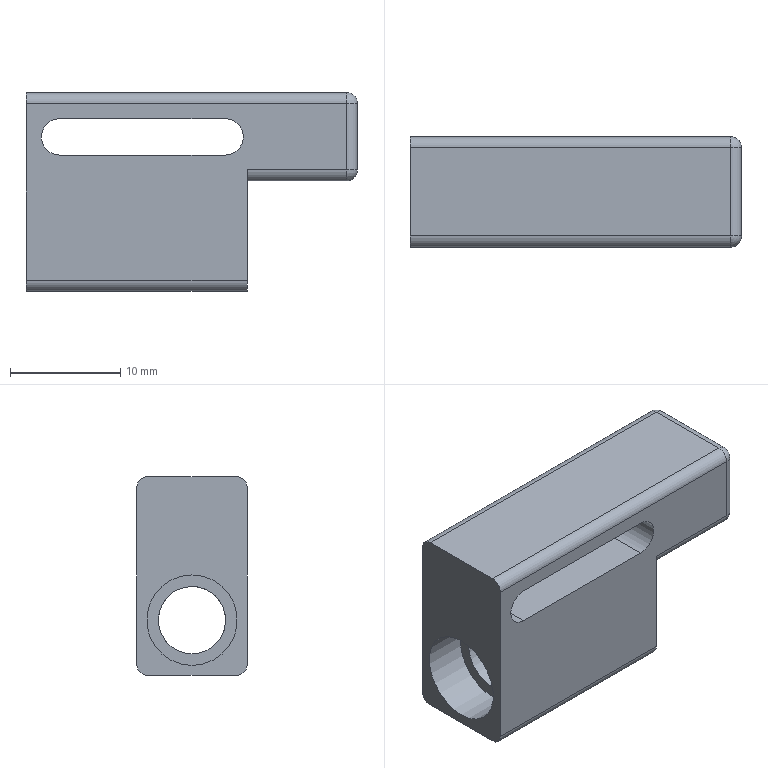Part | NX | 1 solid | 29 faces | box 30 x 10 x 18 mm | volume 3108 mm3 | cylinder 14 | plane 11 | sphere 4 | commonest cylinder face diameters 2 x10 3.3 x2 6.1 x1 8.2 x1
STEP:
#1=CARTESIAN_POINT('',(-11.,5.,-12.05));
#2=VERTEX_POINT('',#1);
#3=CARTESIAN_POINT('',(-11.,5.,-9.));
#4=DIRECTION('',(-1.,0.,0.));
#5=DIRECTION('',(0.,0.,-1.));
#6=AXIS2_PLACEMENT_3D('',#3,#4,#5);
#7=CIRCLE('',#6,3.05);
#8=EDGE_CURVE('',#2,#2,#7,.T.);
#9=ORIENTED_EDGE('',*,*,#8,.F.);
#10=EDGE_LOOP('',(#9));
#11=FACE_BOUND('',#10,.T.);
#12=CARTESIAN_POINT('',(-11.,5.,-13.1));
#13=VERTEX_POINT('',#12);
#14=CARTESIAN_POINT('',(-11.,5.,-9.));
#15=DIRECTION('',(1.,0.,0.));
#16=DIRECTION('',(0.,0.,-1.));
#17=AXIS2_PLACEMENT_3D('',#14,#15,#16);
#18=CIRCLE('',#17,4.1);
#19=EDGE_CURVE('',#13,#13,#18,.T.);
#20=ORIENTED_EDGE('',*,*,#19,.F.);
#21=EDGE_LOOP('',(#20));
#22=FACE_BOUND('',#21,.T.);
#23=CARTESIAN_POINT('',(-11.,5.,-9.));
#24=DIRECTION('',(1.,0.,0.));
#25=DIRECTION('',(0.,0.,-1.));
#26=AXIS2_PLACEMENT_3D('',#23,#24,#25);
#27=PLANE('',#26);
#28=ADVANCED_FACE('',(#11,#22),#27,.F.);
#29=CARTESIAN_POINT('',(5.,0.,-13.));
#30=VERTEX_POINT('',#29);
#31=CARTESIAN_POINT('',(5.,1.,-14.));
#32=VERTEX_POINT('',#31);
#33=CARTESIAN_POINT('',(5.,1.,-13.));
#34=DIRECTION('',(1.,0.,0.));
#35=DIRECTION('',(0.,-1.,0.));
#36=AXIS2_PLACEMENT_3D('',#33,#34,#35);
#37=CIRCLE('',#36,1.);
#38=EDGE_CURVE('',#30,#32,#37,.T.);
#39=ORIENTED_EDGE('',*,*,#38,.F.);
#40=CARTESIAN_POINT('',(-15.,0.,-13.));
#41=VERTEX_POINT('',#40);
#42=CARTESIAN_POINT('',(5.,0.,-13.));
#43=DIRECTION('',(1.,0.,0.));
#44=VECTOR('',#43,1000.);
#45=LINE('',#42,#44);
#46=EDGE_CURVE('',#41,#30,#45,.T.);
#47=ORIENTED_EDGE('',*,*,#46,.F.);
#48=CARTESIAN_POINT('',(-15.,1.,-14.));
#49=VERTEX_POINT('',#48);
#50=CARTESIAN_POINT('',(-15.,1.,-13.));
#51=DIRECTION('',(-1.,0.,0.));
#52=DIRECTION('',(0.,0.,-1.));
#53=AXIS2_PLACEMENT_3D('',#50,#51,#52);
#54=CIRCLE('',#53,1.);
#55=EDGE_CURVE('',#49,#41,#54,.T.);
#56=ORIENTED_EDGE('',*,*,#55,.F.);
#57=CARTESIAN_POINT('',(-15.,1.,-14.));
#58=DIRECTION('',(-1.,0.,0.));
#59=VECTOR('',#58,1000.);
#60=LINE('',#57,#59);
#61=EDGE_CURVE('',#32,#49,#60,.T.);
#62=ORIENTED_EDGE('',*,*,#61,.F.);
#63=EDGE_LOOP('',(#39,#47,#56,#62));
#64=FACE_BOUND('',#63,.T.);
#65=CARTESIAN_POINT('',(0.,1.,-13.));
#66=DIRECTION('',(1.,0.,0.));
#67=DIRECTION('',(0.,0.,-1.));
#68=AXIS2_PLACEMENT_3D('',#65,#66,#67);
#69=CYLINDRICAL_SURFACE('',#68,1.);
#70=ADVANCED_FACE('',(#64),#69,.T.);
#71=CARTESIAN_POINT('',(-15.,10.,-13.));
#72=VERTEX_POINT('',#71);
#73=CARTESIAN_POINT('',(-15.,9.,-14.));
#74=VERTEX_POINT('',#73);
#75=CARTESIAN_POINT('',(-15.,9.,-13.));
#76=DIRECTION('',(-1.,0.,0.));
#77=DIRECTION('',(0.,0.,-1.));
#78=AXIS2_PLACEMENT_3D('',#75,#76,#77);
#79=CIRCLE('',#78,1.);
#80=EDGE_CURVE('',#72,#74,#79,.T.);
#81=ORIENTED_EDGE('',*,*,#80,.F.);
#82=CARTESIAN_POINT('',(5.,10.,-13.));
#83=VERTEX_POINT('',#82);
#84=CARTESIAN_POINT('',(0.,10.,-13.));
#85=DIRECTION('',(-1.,0.,0.));
#86=VECTOR('',#85,1000.);
#87=LINE('',#84,#86);
#88=EDGE_CURVE('',#83,#72,#87,.T.);
#89=ORIENTED_EDGE('',*,*,#88,.F.);
#90=CARTESIAN_POINT('',(5.,9.,-14.));
#91=VERTEX_POINT('',#90);
#92=CARTESIAN_POINT('',(5.,9.,-13.));
#93=DIRECTION('',(1.,0.,0.));
#94=DIRECTION('',(0.,-1.,0.));
#95=AXIS2_PLACEMENT_3D('',#92,#93,#94);
#96=CIRCLE('',#95,1.);
#97=EDGE_CURVE('',#91,#83,#96,.T.);
#98=ORIENTED_EDGE('',*,*,#97,.F.);
#99=CARTESIAN_POINT('',(0.,9.,-14.));
#100=DIRECTION('',(1.,0.,0.));
#101=VECTOR('',#100,1000.);
#102=LINE('',#99,#101);
#103=EDGE_CURVE('',#74,#91,#102,.T.);
#104=ORIENTED_EDGE('',*,*,#103,.F.);
#105=EDGE_LOOP('',(#81,#89,#98,#104));
#106=FACE_BOUND('',#105,.T.);
#107=CARTESIAN_POINT('',(0.,9.,-13.));
#108=DIRECTION('',(1.,0.,0.));
#109=DIRECTION('',(0.,0.,-1.));
#110=AXIS2_PLACEMENT_3D('',#107,#108,#109);
#111=CYLINDRICAL_SURFACE('',#110,1.);
#112=ADVANCED_FACE('',(#106),#111,.T.);
#113=CARTESIAN_POINT('',(15.,1.,3.));
#114=VERTEX_POINT('',#113);
#115=CARTESIAN_POINT('',(14.,1.,4.));
#116=VERTEX_POINT('',#115);
#117=CARTESIAN_POINT('',(14.,1.,3.));
#118=DIRECTION('',(0.,-1.,0.));
#119=DIRECTION('',(0.,0.,-1.));
#120=AXIS2_PLACEMENT_3D('',#117,#118,#119);
#121=CIRCLE('',#120,1.);
#122=EDGE_CURVE('',#114,#116,#121,.T.);
#123=ORIENTED_EDGE('',*,*,#122,.T.);
#124=CARTESIAN_POINT('',(14.,0.,3.));
#125=VERTEX_POINT('',#124);
#126=CARTESIAN_POINT('',(14.,1.,3.));
#127=DIRECTION('',(-1.,0.,0.));
#128=DIRECTION('',(0.,0.,1.));
#129=AXIS2_PLACEMENT_3D('',#126,#127,#128);
#130=CIRCLE('',#129,1.);
#131=EDGE_CURVE('',#125,#116,#130,.T.);
#132=ORIENTED_EDGE('',*,*,#131,.F.);
#133=CARTESIAN_POINT('',(14.,1.,3.));
#134=DIRECTION('',(0.,0.,1.));
#135=DIRECTION('',(1.,0.,0.));
#136=AXIS2_PLACEMENT_3D('',#133,#134,#135);
#137=CIRCLE('',#136,1.);
#138=EDGE_CURVE('',#125,#114,#137,.T.);
#139=ORIENTED_EDGE('',*,*,#138,.T.);
#140=EDGE_LOOP('',(#123,#132,#139));
#141=FACE_BOUND('',#140,.T.);
#142=CARTESIAN_POINT('',(14.,1.,3.));
#143=DIRECTION('',(0.,0.,1.));
#144=DIRECTION('',(1.,0.,0.));
#145=AXIS2_PLACEMENT_3D('',#142,#143,#144);
#146=SPHERICAL_SURFACE('',#145,1.);
#147=ADVANCED_FACE('',(#141),#146,.T.);
#148=CARTESIAN_POINT('',(14.,0.,-3.));
#149=VERTEX_POINT('',#148);
#150=CARTESIAN_POINT('',(15.,1.,-3.));
#151=VERTEX_POINT('',#150);
#152=CARTESIAN_POINT('',(14.,1.,-3.));
#153=DIRECTION('',(0.,0.,1.));
#154=DIRECTION('',(1.,0.,0.));
#155=AXIS2_PLACEMENT_3D('',#152,#153,#154);
#156=CIRCLE('',#155,1.);
#157=EDGE_CURVE('',#149,#151,#156,.T.);
#158=ORIENTED_EDGE('',*,*,#157,.T.);
#159=CARTESIAN_POINT('',(15.,1.,-3.));
#160=DIRECTION('',(0.,0.,-1.));
#161=VECTOR('',#160,1000.);
#162=LINE('',#159,#161);
#163=EDGE_CURVE('',#114,#151,#162,.T.);
#164=ORIENTED_EDGE('',*,*,#163,.F.);
#165=ORIENTED_EDGE('',*,*,#138,.F.);
#166=CARTESIAN_POINT('',(14.,0.,3.));
#167=DIRECTION('',(0.,0.,1.));
#168=VECTOR('',#167,1000.);
#169=LINE('',#166,#168);
#170=EDGE_CURVE('',#149,#125,#169,.T.);
#171=ORIENTED_EDGE('',*,*,#170,.F.);
#172=EDGE_LOOP('',(#158,#164,#165,#171));
#173=FACE_BOUND('',#172,.T.);
#174=CARTESIAN_POINT('',(14.,1.,4.));
#175=DIRECTION('',(0.,0.,1.));
#176=DIRECTION('',(1.,0.,0.));
#177=AXIS2_PLACEMENT_3D('',#174,#175,#176);
#178=CYLINDRICAL_SURFACE('',#177,1.);
#179=ADVANCED_FACE('',(#173),#178,.T.);
#180=CARTESIAN_POINT('',(15.,9.,3.));
#181=VERTEX_POINT('',#180);
#182=CARTESIAN_POINT('',(14.,9.,4.));
#183=VERTEX_POINT('',#182);
#184=CARTESIAN_POINT('',(14.,9.,3.));
#185=DIRECTION('',(0.,-1.,0.));
#186=DIRECTION('',(0.,0.,-1.));
#187=AXIS2_PLACEMENT_3D('',#184,#185,#186);
#188=CIRCLE('',#187,1.);
#189=EDGE_CURVE('',#181,#183,#188,.T.);
#190=ORIENTED_EDGE('',*,*,#189,.T.);
#191=CARTESIAN_POINT('',(14.,10.,4.));
#192=DIRECTION('',(0.,1.,0.));
#193=VECTOR('',#192,1000.);
#194=LINE('',#191,#193);
#195=EDGE_CURVE('',#116,#183,#194,.T.);
#196=ORIENTED_EDGE('',*,*,#195,.F.);
#197=ORIENTED_EDGE('',*,*,#122,.F.);
#198=CARTESIAN_POINT('',(15.,10.,3.));
#199=DIRECTION('',(0.,-1.,0.));
#200=VECTOR('',#199,1000.);
#201=LINE('',#198,#200);
#202=EDGE_CURVE('',#181,#114,#201,.T.);
#203=ORIENTED_EDGE('',*,*,#202,.F.);
#204=EDGE_LOOP('',(#190,#196,#197,#203));
#205=FACE_BOUND('',#204,.T.);
#206=CARTESIAN_POINT('',(14.,10.,3.));
#207=DIRECTION('',(0.,-1.,0.));
#208=DIRECTION('',(0.,0.,-1.));
#209=AXIS2_PLACEMENT_3D('',#206,#207,#208);
#210=CYLINDRICAL_SURFACE('',#209,1.);
#211=ADVANCED_FACE('',(#205),#210,.T.);
#212=CARTESIAN_POINT('',(14.,1.,-4.));
#213=VERTEX_POINT('',#212);
#214=CARTESIAN_POINT('',(14.,1.,-3.));
#215=DIRECTION('',(1.,0.,0.));
#216=DIRECTION('',(0.,0.,-1.));
#217=AXIS2_PLACEMENT_3D('',#214,#215,#216);
#218=CIRCLE('',#217,1.);
#219=EDGE_CURVE('',#213,#149,#218,.F.);
#220=ORIENTED_EDGE('',*,*,#219,.F.);
#221=CARTESIAN_POINT('',(14.,1.,-3.));
#222=DIRECTION('',(0.,-1.,0.));
#223=DIRECTION('',(0.,0.,-1.));
#224=AXIS2_PLACEMENT_3D('',#221,#222,#223);
#225=CIRCLE('',#224,1.);
#226=EDGE_CURVE('',#213,#151,#225,.T.);
#227=ORIENTED_EDGE('',*,*,#226,.T.);
#228=ORIENTED_EDGE('',*,*,#157,.F.);
#229=EDGE_LOOP('',(#220,#227,#228));
#230=FACE_BOUND('',#229,.T.);
#231=CARTESIAN_POINT('',(14.,1.,-3.));
#232=DIRECTION('',(0.,0.,1.));
#233=DIRECTION('',(1.,0.,0.));
#234=AXIS2_PLACEMENT_3D('',#231,#232,#233);
#235=SPHERICAL_SURFACE('',#234,1.);
#236=ADVANCED_FACE('',(#230),#235,.T.);
#237=CARTESIAN_POINT('',(14.,10.,3.));
#238=VERTEX_POINT('',#237);
#239=CARTESIAN_POINT('',(14.,9.,3.));
#240=DIRECTION('',(0.,0.,-1.));
#241=DIRECTION('',(-1.,0.,0.));
#242=AXIS2_PLACEMENT_3D('',#239,#240,#241);
#243=CIRCLE('',#242,1.);
#244=EDGE_CURVE('',#181,#238,#243,.F.);
#245=ORIENTED_EDGE('',*,*,#244,.T.);
#246=CARTESIAN_POINT('',(14.,9.,3.));
#247=DIRECTION('',(1.,0.,0.));
#248=DIRECTION('',(0.,0.,-1.));
#249=AXIS2_PLACEMENT_3D('',#246,#247,#248);
#250=CIRCLE('',#249,1.);
#251=EDGE_CURVE('',#183,#238,#250,.F.);
#252=ORIENTED_EDGE('',*,*,#251,.F.);
#253=ORIENTED_EDGE('',*,*,#189,.F.);
#254=EDGE_LOOP('',(#245,#252,#253));
#255=FACE_BOUND('',#254,.T.);
#256=CARTESIAN_POINT('',(14.,9.,3.));
#257=DIRECTION('',(0.,0.,1.));
#258=DIRECTION('',(1.,0.,0.));
#259=AXIS2_PLACEMENT_3D('',#256,#257,#258);
#260=SPHERICAL_SURFACE('',#259,1.);
#261=ADVANCED_FACE('',(#255),#260,.T.);
#262=CARTESIAN_POINT('',(14.,9.,-4.));
#263=VERTEX_POINT('',#262);
#264=CARTESIAN_POINT('',(15.,9.,-3.));
#265=VERTEX_POINT('',#264);
#266=CARTESIAN_POINT('',(14.,9.,-3.));
#267=DIRECTION('',(0.,-1.,0.));
#268=DIRECTION('',(0.,0.,-1.));
#269=AXIS2_PLACEMENT_3D('',#266,#267,#268);
#270=CIRCLE('',#269,1.);
#271=EDGE_CURVE('',#263,#265,#270,.T.);
#272=ORIENTED_EDGE('',*,*,#271,.T.);
#273=CARTESIAN_POINT('',(15.,10.,-3.));
#274=DIRECTION('',(0.,1.,0.));
#275=VECTOR('',#274,1000.);
#276=LINE('',#273,#275);
#277=EDGE_CURVE('',#151,#265,#276,.T.);
#278=ORIENTED_EDGE('',*,*,#277,.F.);
#279=ORIENTED_EDGE('',*,*,#226,.F.);
#280=CARTESIAN_POINT('',(14.,10.,-4.));
#281=DIRECTION('',(0.,-1.,0.));
#282=VECTOR('',#281,1000.);
#283=LINE('',#280,#282);
#284=EDGE_CURVE('',#263,#213,#283,.T.);
#285=ORIENTED_EDGE('',*,*,#284,.F.);
#286=EDGE_LOOP('',(#272,#278,#279,#285));
#287=FACE_BOUND('',#286,.T.);
#288=CARTESIAN_POINT('',(14.,10.,-3.));
#289=DIRECTION('',(0.,-1.,0.));
#290=DIRECTION('',(0.,0.,-1.));
#291=AXIS2_PLACEMENT_3D('',#288,#289,#290);
#292=CYLINDRICAL_SURFACE('',#291,1.);
#293=ADVANCED_FACE('',(#287),#292,.T.);
#294=CARTESIAN_POINT('',(14.,10.,-3.));
#295=VERTEX_POINT('',#294);
#296=CARTESIAN_POINT('',(14.,9.,-3.));
#297=DIRECTION('',(0.,0.,-1.));
#298=DIRECTION('',(-1.,0.,0.));
#299=AXIS2_PLACEMENT_3D('',#296,#297,#298);
#300=CIRCLE('',#299,1.);
#301=EDGE_CURVE('',#265,#295,#300,.F.);
#302=ORIENTED_EDGE('',*,*,#301,.T.);
#303=CARTESIAN_POINT('',(14.,10.,0.));
#304=DIRECTION('',(0.,0.,-1.));
#305=VECTOR('',#304,1000.);
#306=LINE('',#303,#305);
#307=EDGE_CURVE('',#238,#295,#306,.T.);
#308=ORIENTED_EDGE('',*,*,#307,.F.);
#309=ORIENTED_EDGE('',*,*,#244,.F.);
#310=CARTESIAN_POINT('',(15.,9.,4.));
#311=DIRECTION('',(0.,0.,1.));
#312=VECTOR('',#311,1000.);
#313=LINE('',#310,#312);
#314=EDGE_CURVE('',#265,#181,#313,.T.);
#315=ORIENTED_EDGE('',*,*,#314,.F.);
#316=EDGE_LOOP('',(#302,#308,#309,#315));
#317=FACE_BOUND('',#316,.T.);
#318=CARTESIAN_POINT('',(14.,9.,0.));
#319=DIRECTION('',(0.,0.,-1.));
#320=DIRECTION('',(-1.,0.,0.));
#321=AXIS2_PLACEMENT_3D('',#318,#319,#320);
#322=CYLINDRICAL_SURFACE('',#321,1.);
#323=ADVANCED_FACE('',(#317),#322,.T.);
#324=ORIENTED_EDGE('',*,*,#271,.F.);
#325=CARTESIAN_POINT('',(14.,9.,-3.));
#326=DIRECTION('',(-1.,0.,0.));
#327=DIRECTION('',(0.,0.,1.));
#328=AXIS2_PLACEMENT_3D('',#325,#326,#327);
#329=CIRCLE('',#328,1.);
#330=EDGE_CURVE('',#295,#263,#329,.T.);
#331=ORIENTED_EDGE('',*,*,#330,.F.);
#332=ORIENTED_EDGE('',*,*,#301,.F.);
#333=EDGE_LOOP('',(#324,#331,#332));
#334=FACE_BOUND('',#333,.T.);
#335=CARTESIAN_POINT('',(14.,9.,-3.));
#336=DIRECTION('',(0.,0.,1.));
#337=DIRECTION('',(1.,0.,0.));
#338=AXIS2_PLACEMENT_3D('',#335,#336,#337);
#339=SPHERICAL_SURFACE('',#338,1.);
#340=ADVANCED_FACE('',(#334),#339,.T.);
#341=CARTESIAN_POINT('',(-15.,0.,3.));
#342=VERTEX_POINT('',#341);
#343=CARTESIAN_POINT('',(-15.,0.,3.));
#344=DIRECTION('',(-1.,0.,0.));
#345=VECTOR('',#344,1000.);
#346=LINE('',#343,#345);
#347=EDGE_CURVE('',#125,#342,#346,.T.);
#348=ORIENTED_EDGE('',*,*,#347,.F.);
#349=ORIENTED_EDGE('',*,*,#131,.T.);
#350=CARTESIAN_POINT('',(-15.,1.,4.));
#351=VERTEX_POINT('',#350);
#352=CARTESIAN_POINT('',(15.,1.,4.));
#353=DIRECTION('',(1.,0.,0.));
#354=VECTOR('',#353,1000.);
#355=LINE('',#352,#354);
#356=EDGE_CURVE('',#351,#116,#355,.T.);
#357=ORIENTED_EDGE('',*,*,#356,.F.);
#358=CARTESIAN_POINT('',(-15.,1.,3.));
#359=DIRECTION('',(-1.,0.,0.));
#360=DIRECTION('',(0.,0.,-1.));
#361=AXIS2_PLACEMENT_3D('',#358,#359,#360);
#362=CIRCLE('',#361,1.);
#363=EDGE_CURVE('',#342,#351,#362,.T.);
#364=ORIENTED_EDGE('',*,*,#363,.F.);
#365=EDGE_LOOP('',(#348,#349,#357,#364));
#366=FACE_BOUND('',#365,.T.);
#367=CARTESIAN_POINT('',(-15.,1.,3.));
#368=DIRECTION('',(-1.,0.,0.));
#369=DIRECTION('',(0.,0.,1.));
#370=AXIS2_PLACEMENT_3D('',#367,#368,#369);
#371=CYLINDRICAL_SURFACE('',#370,1.);
#372=ADVANCED_FACE('',(#366),#371,.T.);
#373=CARTESIAN_POINT('',(-15.,9.,4.));
#374=VERTEX_POINT('',#373);
#375=CARTESIAN_POINT('',(-15.,9.,4.));
#376=DIRECTION('',(-1.,0.,0.));
#377=VECTOR('',#376,1000.);
#378=LINE('',#375,#377);
#379=EDGE_CURVE('',#183,#374,#378,.T.);
#380=ORIENTED_EDGE('',*,*,#379,.F.);
#381=ORIENTED_EDGE('',*,*,#251,.T.);
#382=CARTESIAN_POINT('',(-15.,10.,3.));
#383=VERTEX_POINT('',#382);
#384=CARTESIAN_POINT('',(0.,10.,3.));
#385=DIRECTION('',(1.,0.,0.));
#386=VECTOR('',#385,1000.);
#387=LINE('',#384,#386);
#388=EDGE_CURVE('',#383,#238,#387,.T.);
#389=ORIENTED_EDGE('',*,*,#388,.F.);
#390=CARTESIAN_POINT('',(-15.,9.,3.));
#391=DIRECTION('',(-1.,0.,0.));
#392=DIRECTION('',(0.,0.,-1.));
#393=AXIS2_PLACEMENT_3D('',#390,#391,#392);
#394=CIRCLE('',#393,1.);
#395=EDGE_CURVE('',#374,#383,#394,.T.);
#396=ORIENTED_EDGE('',*,*,#395,.F.);
#397=EDGE_LOOP('',(#380,#381,#389,#396));
#398=FACE_BOUND('',#397,.T.);
#399=CARTESIAN_POINT('',(0.,9.,3.));
#400=DIRECTION('',(1.,0.,0.));
#401=DIRECTION('',(0.,0.,-1.));
#402=AXIS2_PLACEMENT_3D('',#399,#400,#401);
#403=CYLINDRICAL_SURFACE('',#402,1.);
#404=ADVANCED_FACE('',(#398),#403,.T.);
#405=CARTESIAN_POINT('',(5.,1.,-4.));
#406=VERTEX_POINT('',#405);
#407=CARTESIAN_POINT('',(5.,1.,-4.));
#408=DIRECTION('',(-1.,0.,0.));
#409=VECTOR('',#408,1000.);
#410=LINE('',#407,#409);
#411=EDGE_CURVE('',#213,#406,#410,.T.);
#412=ORIENTED_EDGE('',*,*,#411,.F.);
#413=ORIENTED_EDGE('',*,*,#219,.T.);
#414=CARTESIAN_POINT('',(5.,0.,-3.));
#415=VERTEX_POINT('',#414);
#416=CARTESIAN_POINT('',(15.,0.,-3.));
#417=DIRECTION('',(1.,0.,0.));
#418=VECTOR('',#417,1000.);
#419=LINE('',#416,#418);
#420=EDGE_CURVE('',#415,#149,#419,.T.);
#421=ORIENTED_EDGE('',*,*,#420,.F.);
#422=CARTESIAN_POINT('',(5.,1.,-3.));
#423=DIRECTION('',(-1.,0.,0.));
#424=DIRECTION('',(0.,-1.,0.));
#425=AXIS2_PLACEMENT_3D('',#422,#423,#424);
#426=CIRCLE('',#425,1.);
#427=EDGE_CURVE('',#406,#415,#426,.T.);
#428=ORIENTED_EDGE('',*,*,#427,.F.);
#429=EDGE_LOOP('',(#412,#413,#421,#428));
#430=FACE_BOUND('',#429,.T.);
#431=CARTESIAN_POINT('',(-15.,1.,-3.));
#432=DIRECTION('',(1.,0.,0.));
#433=DIRECTION('',(0.,0.,-1.));
#434=AXIS2_PLACEMENT_3D('',#431,#432,#433);
#435=CYLINDRICAL_SURFACE('',#434,1.);
#436=ADVANCED_FACE('',(#430),#435,.T.);
#437=CARTESIAN_POINT('',(5.,10.,-3.));
#438=VERTEX_POINT('',#437);
#439=CARTESIAN_POINT('',(0.,10.,-3.));
#440=DIRECTION('',(-1.,0.,0.));
#441=VECTOR('',#440,1000.);
#442=LINE('',#439,#441);
#443=EDGE_CURVE('',#295,#438,#442,.T.);
#444=ORIENTED_EDGE('',*,*,#443,.F.);
#445=ORIENTED_EDGE('',*,*,#330,.T.);
#446=CARTESIAN_POINT('',(5.,9.,-4.));
#447=VERTEX_POINT('',#446);
#448=CARTESIAN_POINT('',(-15.,9.,-4.));
#449=DIRECTION('',(1.,0.,0.));
#450=VECTOR('',#449,1000.);
#451=LINE('',#448,#450);
#452=EDGE_CURVE('',#447,#263,#451,.T.);
#453=ORIENTED_EDGE('',*,*,#452,.F.);
#454=CARTESIAN_POINT('',(5.,9.,-3.));
#455=DIRECTION('',(-1.,0.,0.));
#456=DIRECTION('',(0.,-1.,0.));
#457=AXIS2_PLACEMENT_3D('',#454,#455,#456);
#458=CIRCLE('',#457,1.);
#459=EDGE_CURVE('',#438,#447,#458,.T.);
#460=ORIENTED_EDGE('',*,*,#459,.F.);
#461=EDGE_LOOP('',(#444,#445,#453,#460));
#462=FACE_BOUND('',#461,.T.);
#463=CARTESIAN_POINT('',(0.,9.,-3.));
#464=DIRECTION('',(-1.,0.,0.));
#465=DIRECTION('',(0.,0.,1.));
#466=AXIS2_PLACEMENT_3D('',#463,#464,#465);
#467=CYLINDRICAL_SURFACE('',#466,1.);
#468=ADVANCED_FACE('',(#462),#467,.T.);
#469=CARTESIAN_POINT('',(-15.,10.,-14.));
#470=DIRECTION('',(0.,1.,0.));
#471=VECTOR('',#470,1000.);
#472=LINE('',#469,#471);
#473=EDGE_CURVE('',#49,#74,#472,.T.);
#474=ORIENTED_EDGE('',*,*,#473,.T.);
#475=ORIENTED_EDGE('',*,*,#103,.T.);
#476=CARTESIAN_POINT('',(5.,10.,-14.));
#477=DIRECTION('',(0.,-1.,0.));
#478=VECTOR('',#477,1000.);
#479=LINE('',#476,#478);
#480=EDGE_CURVE('',#91,#32,#479,.T.);
#481=ORIENTED_EDGE('',*,*,#480,.T.);
#482=ORIENTED_EDGE('',*,*,#61,.T.);
#483=EDGE_LOOP('',(#474,#475,#481,#482));
#484=FACE_BOUND('',#483,.T.);
#485=CARTESIAN_POINT('',(0.,0.,-14.));
#486=DIRECTION('',(0.,0.,1.));
#487=DIRECTION('',(1.,0.,0.));
#488=AXIS2_PLACEMENT_3D('',#485,#486,#487);
#489=PLANE('',#488);
#490=ADVANCED_FACE('',(#484),#489,.F.);
#491=ORIENTED_EDGE('',*,*,#480,.F.);
#492=ORIENTED_EDGE('',*,*,#97,.T.);
#493=CARTESIAN_POINT('',(5.,10.,-14.));
#494=DIRECTION('',(0.,0.,1.));
#495=VECTOR('',#494,1000.);
#496=LINE('',#493,#495);
#497=EDGE_CURVE('',#83,#438,#496,.T.);
#498=ORIENTED_EDGE('',*,*,#497,.T.);
#499=ORIENTED_EDGE('',*,*,#459,.T.);
#500=CARTESIAN_POINT('',(5.,10.,-4.));
#501=DIRECTION('',(0.,-1.,0.));
#502=VECTOR('',#501,1000.);
#503=LINE('',#500,#502);
#504=EDGE_CURVE('',#447,#406,#503,.T.);
#505=ORIENTED_EDGE('',*,*,#504,.T.);
#506=ORIENTED_EDGE('',*,*,#427,.T.);
#507=CARTESIAN_POINT('',(5.,0.,-14.));
#508=DIRECTION('',(0.,0.,1.));
#509=VECTOR('',#508,1000.);
#510=LINE('',#507,#509);
#511=EDGE_CURVE('',#30,#415,#510,.T.);
#512=ORIENTED_EDGE('',*,*,#511,.F.);
#513=ORIENTED_EDGE('',*,*,#38,.T.);
#514=EDGE_LOOP('',(#491,#492,#498,#499,#505,#506,#512,#513));
#515=FACE_BOUND('',#514,.T.);
#516=CARTESIAN_POINT('',(5.,8.05,-9.));
#517=VERTEX_POINT('',#516);
#518=CARTESIAN_POINT('',(5.,5.,-9.));
#519=DIRECTION('',(1.,0.,0.));
#520=DIRECTION('',(0.,1.,0.));
#521=AXIS2_PLACEMENT_3D('',#518,#519,#520);
#522=CIRCLE('',#521,3.05);
#523=EDGE_CURVE('',#517,#517,#522,.T.);
#524=ORIENTED_EDGE('',*,*,#523,.F.);
#525=EDGE_LOOP('',(#524));
#526=FACE_BOUND('',#525,.T.);
#527=CARTESIAN_POINT('',(5.,10.,-14.));
#528=DIRECTION('',(-1.,0.,0.));
#529=DIRECTION('',(0.,-1.,0.));
#530=AXIS2_PLACEMENT_3D('',#527,#528,#529);
#531=PLANE('',#530);
#532=ADVANCED_FACE('',(#515,#526),#531,.F.);
#533=CARTESIAN_POINT('',(3.,0.,1.65));
#534=VERTEX_POINT('',#533);
#535=CARTESIAN_POINT('',(-12.,0.,1.65));
#536=VERTEX_POINT('',#535);
#537=CARTESIAN_POINT('',(0.,0.,1.65));
#538=DIRECTION('',(-1.,0.,0.));
#539=VECTOR('',#538,1000.);
#540=LINE('',#537,#539);
#541=EDGE_CURVE('',#534,#536,#540,.T.);
#542=ORIENTED_EDGE('',*,*,#541,.T.);
#543=CARTESIAN_POINT('',(-12.,10.,1.65));
#544=VERTEX_POINT('',#543);
#545=CARTESIAN_POINT('',(-12.,-101.,1.65));
#546=DIRECTION('',(0.,1.,0.));
#547=VECTOR('',#546,1000.);
#548=LINE('',#545,#547);
#549=EDGE_CURVE('',#536,#544,#548,.T.);
#550=ORIENTED_EDGE('',*,*,#549,.T.);
#551=CARTESIAN_POINT('',(3.,10.,1.65));
#552=VERTEX_POINT('',#551);
#553=CARTESIAN_POINT('',(-12.,10.,1.65));
#554=DIRECTION('',(1.,0.,0.));
#555=VECTOR('',#554,1000.);
#556=LINE('',#553,#555);
#557=EDGE_CURVE('',#544,#552,#556,.T.);
#558=ORIENTED_EDGE('',*,*,#557,.T.);
#559=CARTESIAN_POINT('',(3.,-101.,1.65));
#560=DIRECTION('',(0.,1.,0.));
#561=VECTOR('',#560,1000.);
#562=LINE('',#559,#561);
#563=EDGE_CURVE('',#534,#552,#562,.T.);
#564=ORIENTED_EDGE('',*,*,#563,.F.);
#565=EDGE_LOOP('',(#542,#550,#558,#564));
#566=FACE_BOUND('',#565,.T.);
#567=CARTESIAN_POINT('',(-12.,-101.,1.65));
#568=DIRECTION('',(0.,0.,1.));
#569=DIRECTION('',(1.,0.,0.));
#570=AXIS2_PLACEMENT_3D('',#567,#568,#569);
#571=PLANE('',#570);
#572=ADVANCED_FACE('',(#566),#571,.F.);
#573=CARTESIAN_POINT('',(3.,0.,-1.65));
#574=VERTEX_POINT('',#573);
#575=CARTESIAN_POINT('',(3.,0.,0.));
#576=DIRECTION('',(0.,-1.,0.));
#577=DIRECTION('',(0.,0.,-1.));
#578=AXIS2_PLACEMENT_3D('',#575,#576,#577);
#579=CIRCLE('',#578,1.65);
#580=EDGE_CURVE('',#574,#534,#579,.T.);
#581=ORIENTED_EDGE('',*,*,#580,.T.);
#582=ORIENTED_EDGE('',*,*,#563,.T.);
#583=CARTESIAN_POINT('',(3.,10.,-1.65));
#584=VERTEX_POINT('',#583);
#585=CARTESIAN_POINT('',(3.,10.,0.));
#586=DIRECTION('',(0.,1.,0.));
#587=DIRECTION('',(0.,0.,1.));
#588=AXIS2_PLACEMENT_3D('',#585,#586,#587);
#589=CIRCLE('',#588,1.65);
#590=EDGE_CURVE('',#552,#584,#589,.T.);
#591=ORIENTED_EDGE('',*,*,#590,.T.);
#592=CARTESIAN_POINT('',(3.,-101.,-1.65));
#593=DIRECTION('',(0.,1.,0.));
#594=VECTOR('',#593,1000.);
#595=LINE('',#592,#594);
#596=EDGE_CURVE('',#574,#584,#595,.T.);
#597=ORIENTED_EDGE('',*,*,#596,.F.);
#598=EDGE_LOOP('',(#581,#582,#591,#597));
#599=FACE_BOUND('',#598,.T.);
#600=CARTESIAN_POINT('',(3.,-101.,0.));
#601=DIRECTION('',(0.,1.,0.));
#602=DIRECTION('',(0.,0.,1.));
#603=AXIS2_PLACEMENT_3D('',#600,#601,#602);
#604=CYLINDRICAL_SURFACE('',#603,1.65);
#605=ADVANCED_FACE('',(#599),#604,.F.);
#606=CARTESIAN_POINT('',(-12.,0.,-1.65));
#607=VERTEX_POINT('',#606);
#608=CARTESIAN_POINT('',(0.,0.,-1.65));
#609=DIRECTION('',(1.,0.,0.));
#610=VECTOR('',#609,1000.);
#611=LINE('',#608,#610);
#612=EDGE_CURVE('',#607,#574,#611,.T.);
#613=ORIENTED_EDGE('',*,*,#612,.T.);
#614=ORIENTED_EDGE('',*,*,#596,.T.);
#615=CARTESIAN_POINT('',(-12.,10.,-1.65));
#616=VERTEX_POINT('',#615);
#617=CARTESIAN_POINT('',(-12.,10.,-1.65));
#618=DIRECTION('',(-1.,0.,0.));
#619=VECTOR('',#618,1000.);
#620=LINE('',#617,#619);
#621=EDGE_CURVE('',#584,#616,#620,.T.);
#622=ORIENTED_EDGE('',*,*,#621,.T.);
#623=CARTESIAN_POINT('',(-12.,-101.,-1.65));
#624=DIRECTION('',(0.,1.,0.));
#625=VECTOR('',#624,1000.);
#626=LINE('',#623,#625);
#627=EDGE_CURVE('',#607,#616,#626,.T.);
#628=ORIENTED_EDGE('',*,*,#627,.F.);
#629=EDGE_LOOP('',(#613,#614,#622,#628));
#630=FACE_BOUND('',#629,.T.);
#631=CARTESIAN_POINT('',(-12.,-101.,-1.65));
#632=DIRECTION('',(0.,0.,-1.));
#633=DIRECTION('',(-1.,0.,0.));
#634=AXIS2_PLACEMENT_3D('',#631,#632,#633);
#635=PLANE('',#634);
#636=ADVANCED_FACE('',(#630),#635,.F.);
#637=CARTESIAN_POINT('',(-12.,0.,0.));
#638=DIRECTION('',(0.,-1.,0.));
#639=DIRECTION('',(0.,0.,-1.));
#640=AXIS2_PLACEMENT_3D('',#637,#638,#639);
#641=CIRCLE('',#640,1.65);
#642=EDGE_CURVE('',#536,#607,#641,.T.);
#643=ORIENTED_EDGE('',*,*,#642,.T.);
#644=ORIENTED_EDGE('',*,*,#627,.T.);
#645=CARTESIAN_POINT('',(-12.,10.,0.));
#646=DIRECTION('',(0.,1.,0.));
#647=DIRECTION('',(0.,0.,1.));
#648=AXIS2_PLACEMENT_3D('',#645,#646,#647);
#649=CIRCLE('',#648,1.65);
#650=EDGE_CURVE('',#616,#544,#649,.T.);
#651=ORIENTED_EDGE('',*,*,#650,.T.);
#652=ORIENTED_EDGE('',*,*,#549,.F.);
#653=EDGE_LOOP('',(#643,#644,#651,#652));
#654=FACE_BOUND('',#653,.T.);
#655=CARTESIAN_POINT('',(-12.,-101.,0.));
#656=DIRECTION('',(0.,1.,0.));
#657=DIRECTION('',(0.,0.,1.));
#658=AXIS2_PLACEMENT_3D('',#655,#656,#657);
#659=CYLINDRICAL_SURFACE('',#658,1.65);
#660=ADVANCED_FACE('',(#654),#659,.F.);
#661=CARTESIAN_POINT('',(-15.,0.,4.));
#662=DIRECTION('',(0.,0.,1.));
#663=VECTOR('',#662,1000.);
#664=LINE('',#661,#663);
#665=EDGE_CURVE('',#41,#342,#664,.T.);
#666=ORIENTED_EDGE('',*,*,#665,.F.);
#667=ORIENTED_EDGE('',*,*,#46,.T.);
#668=ORIENTED_EDGE('',*,*,#511,.T.);
#669=ORIENTED_EDGE('',*,*,#420,.T.);
#670=ORIENTED_EDGE('',*,*,#170,.T.);
#671=ORIENTED_EDGE('',*,*,#347,.T.);
#672=EDGE_LOOP('',(#666,#667,#668,#669,#670,#671));
#673=FACE_BOUND('',#672,.T.);
#674=ORIENTED_EDGE('',*,*,#642,.F.);
#675=ORIENTED_EDGE('',*,*,#541,.F.);
#676=ORIENTED_EDGE('',*,*,#580,.F.);
#677=ORIENTED_EDGE('',*,*,#612,.F.);
#678=EDGE_LOOP('',(#674,#675,#676,#677));
#679=FACE_BOUND('',#678,.T.);
#680=CARTESIAN_POINT('',(0.,0.,0.));
#681=DIRECTION('',(0.,-1.,0.));
#682=DIRECTION('',(0.,0.,-1.));
#683=AXIS2_PLACEMENT_3D('',#680,#681,#682);
#684=PLANE('',#683);
#685=ADVANCED_FACE('',(#673,#679),#684,.T.);
#686=ORIENTED_EDGE('',*,*,#497,.F.);
#687=ORIENTED_EDGE('',*,*,#88,.T.);
#688=CARTESIAN_POINT('',(-15.,10.,4.));
#689=DIRECTION('',(0.,0.,1.));
#690=VECTOR('',#689,1000.);
#691=LINE('',#688,#690);
#692=EDGE_CURVE('',#72,#383,#691,.T.);
#693=ORIENTED_EDGE('',*,*,#692,.T.);
#694=ORIENTED_EDGE('',*,*,#388,.T.);
#695=ORIENTED_EDGE('',*,*,#307,.T.);
#696=ORIENTED_EDGE('',*,*,#443,.T.);
#697=EDGE_LOOP('',(#686,#687,#693,#694,#695,#696));
#698=FACE_BOUND('',#697,.T.);
#699=ORIENTED_EDGE('',*,*,#557,.F.);
#700=ORIENTED_EDGE('',*,*,#650,.F.);
#701=ORIENTED_EDGE('',*,*,#621,.F.);
#702=ORIENTED_EDGE('',*,*,#590,.F.);
#703=EDGE_LOOP('',(#699,#700,#701,#702));
#704=FACE_BOUND('',#703,.T.);
#705=CARTESIAN_POINT('',(0.,10.,0.));
#706=DIRECTION('',(0.,-1.,0.));
#707=DIRECTION('',(0.,0.,-1.));
#708=AXIS2_PLACEMENT_3D('',#705,#706,#707);
#709=PLANE('',#708);
#710=ADVANCED_FACE('',(#698,#704),#709,.F.);
#711=ORIENTED_EDGE('',*,*,#356,.T.);
#712=ORIENTED_EDGE('',*,*,#195,.T.);
#713=ORIENTED_EDGE('',*,*,#379,.T.);
#714=CARTESIAN_POINT('',(-15.,10.,4.));
#715=DIRECTION('',(0.,-1.,0.));
#716=VECTOR('',#715,1000.);
#717=LINE('',#714,#716);
#718=EDGE_CURVE('',#374,#351,#717,.T.);
#719=ORIENTED_EDGE('',*,*,#718,.T.);
#720=EDGE_LOOP('',(#711,#712,#713,#719));
#721=FACE_BOUND('',#720,.T.);
#722=CARTESIAN_POINT('',(-15.,10.,4.));
#723=DIRECTION('',(0.,0.,-1.));
#724=DIRECTION('',(-1.,0.,0.));
#725=AXIS2_PLACEMENT_3D('',#722,#723,#724);
#726=PLANE('',#725);
#727=ADVANCED_FACE('',(#721),#726,.F.);
#728=ORIENTED_EDGE('',*,*,#692,.F.);
#729=ORIENTED_EDGE('',*,*,#80,.T.);
#730=ORIENTED_EDGE('',*,*,#473,.F.);
#731=ORIENTED_EDGE('',*,*,#55,.T.);
#732=ORIENTED_EDGE('',*,*,#665,.T.);
#733=ORIENTED_EDGE('',*,*,#363,.T.);
#734=ORIENTED_EDGE('',*,*,#718,.F.);
#735=ORIENTED_EDGE('',*,*,#395,.T.);
#736=EDGE_LOOP('',(#728,#729,#730,#731,#732,#733,#734,#735));
#737=FACE_BOUND('',#736,.T.);
#738=CARTESIAN_POINT('',(-15.,5.,-13.1));
#739=VERTEX_POINT('',#738);
#740=CARTESIAN_POINT('',(-15.,5.,-9.));
#741=DIRECTION('',(1.,0.,0.));
#742=DIRECTION('',(0.,0.,-1.));
#743=AXIS2_PLACEMENT_3D('',#740,#741,#742);
#744=CIRCLE('',#743,4.1);
#745=EDGE_CURVE('',#739,#739,#744,.T.);
#746=ORIENTED_EDGE('',*,*,#745,.T.);
#747=EDGE_LOOP('',(#746));
#748=FACE_BOUND('',#747,.T.);
#749=CARTESIAN_POINT('',(-15.,10.,4.));
#750=DIRECTION('',(1.,0.,0.));
#751=DIRECTION('',(0.,0.,-1.));
#752=AXIS2_PLACEMENT_3D('',#749,#750,#751);
#753=PLANE('',#752);
#754=ADVANCED_FACE('',(#737,#748),#753,.F.);
#755=ORIENTED_EDGE('',*,*,#314,.T.);
#756=ORIENTED_EDGE('',*,*,#202,.T.);
#757=ORIENTED_EDGE('',*,*,#163,.T.);
#758=ORIENTED_EDGE('',*,*,#277,.T.);
#759=EDGE_LOOP('',(#755,#756,#757,#758));
#760=FACE_BOUND('',#759,.T.);
#761=CARTESIAN_POINT('',(15.,10.,4.));
#762=DIRECTION('',(-1.,0.,0.));
#763=DIRECTION('',(0.,0.,1.));
#764=AXIS2_PLACEMENT_3D('',#761,#762,#763);
#765=PLANE('',#764);
#766=ADVANCED_FACE('',(#760),#765,.F.);
#767=ORIENTED_EDGE('',*,*,#452,.T.);
#768=ORIENTED_EDGE('',*,*,#284,.T.);
#769=ORIENTED_EDGE('',*,*,#411,.T.);
#770=ORIENTED_EDGE('',*,*,#504,.F.);
#771=EDGE_LOOP('',(#767,#768,#769,#770));
#772=FACE_BOUND('',#771,.T.);
#773=CARTESIAN_POINT('',(-15.,10.,-4.));
#774=DIRECTION('',(0.,0.,1.));
#775=DIRECTION('',(1.,0.,0.));
#776=AXIS2_PLACEMENT_3D('',#773,#774,#775);
#777=PLANE('',#776);
#778=ADVANCED_FACE('',(#772),#777,.F.);
#779=ORIENTED_EDGE('',*,*,#8,.T.);
#780=EDGE_LOOP('',(#779));
#781=FACE_BOUND('',#780,.T.);
#782=ORIENTED_EDGE('',*,*,#523,.T.);
#783=EDGE_LOOP('',(#782));
#784=FACE_BOUND('',#783,.T.);
#785=CARTESIAN_POINT('',(-15.,5.,-9.));
#786=DIRECTION('',(1.,0.,0.));
#787=DIRECTION('',(0.,1.,0.));
#788=AXIS2_PLACEMENT_3D('',#785,#786,#787);
#789=CYLINDRICAL_SURFACE('',#788,3.05);
#790=ADVANCED_FACE('',(#781,#784),#789,.F.);
#791=ORIENTED_EDGE('',*,*,#19,.T.);
#792=EDGE_LOOP('',(#791));
#793=FACE_BOUND('',#792,.T.);
#794=ORIENTED_EDGE('',*,*,#745,.F.);
#795=EDGE_LOOP('',(#794));
#796=FACE_BOUND('',#795,.T.);
#797=CARTESIAN_POINT('',(-11.,5.,-9.));
#798=DIRECTION('',(-1.,0.,0.));
#799=DIRECTION('',(0.,0.,1.));
#800=AXIS2_PLACEMENT_3D('',#797,#798,#799);
#801=CYLINDRICAL_SURFACE('',#800,4.1);
#802=ADVANCED_FACE('',(#793,#796),#801,.F.);
#803=CLOSED_SHELL('',(#28,#70,#112,#147,#179,#211,#236,#261,#293,#323,#340,#372,#404,#436,#468,#490,#532,#572,#605,#636,#660,#685,#710,#727,#754,#766,#778,#790,#802));
#804=MANIFOLD_SOLID_BREP('',#803);
#805=(LENGTH_UNIT()NAMED_UNIT(*)SI_UNIT(.MILLI.,.METRE.));
#806=UNCERTAINTY_MEASURE_WITH_UNIT(LENGTH_MEASURE(0.00001),#805,'','');
#807=(NAMED_UNIT(*)PLANE_ANGLE_UNIT()SI_UNIT($,.RADIAN.));
#808=(NAMED_UNIT(*)SI_UNIT($,.STERADIAN.)SOLID_ANGLE_UNIT());
#809=(GEOMETRIC_REPRESENTATION_CONTEXT(3)GLOBAL_UNCERTAINTY_ASSIGNED_CONTEXT((#806))GLOBAL_UNIT_ASSIGNED_CONTEXT((#805,#807,#808))REPRESENTATION_CONTEXT('',''));
#810=ADVANCED_BREP_SHAPE_REPRESENTATION('',(#804),#809);